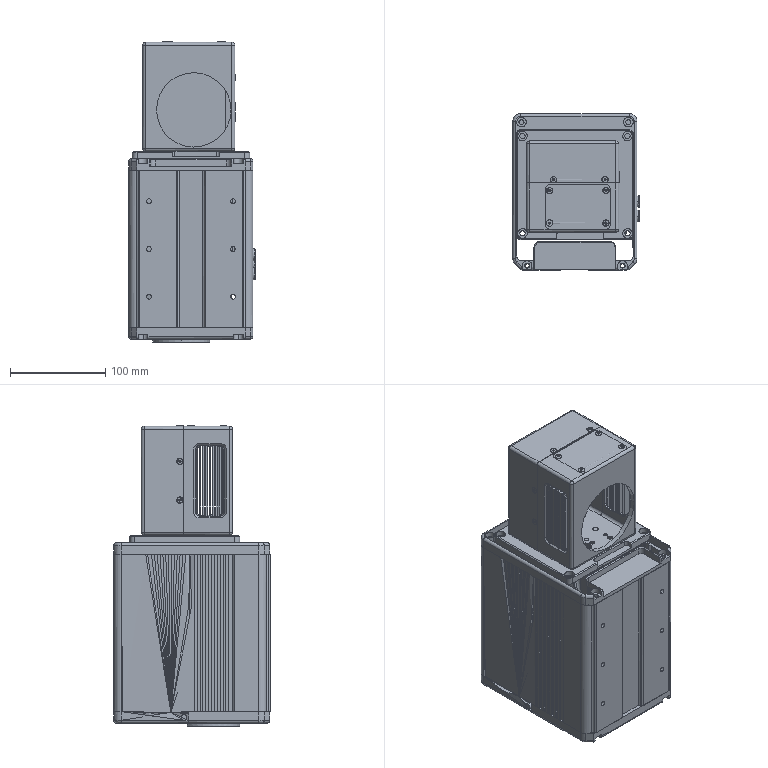Part | NX | features BREP 12 | 2 solids | 826 faces | box 132.2 x 164 x 314.369 mm | volume 1764248 mm3 | plane 476 | cylinder 233 | cone 77 | torus 21 | spline 11 | sphere 8 | commonest cylinder face diameters 6 x54 10 x32 6.72 x20 8 x20 3.2 x17 4.2 x12